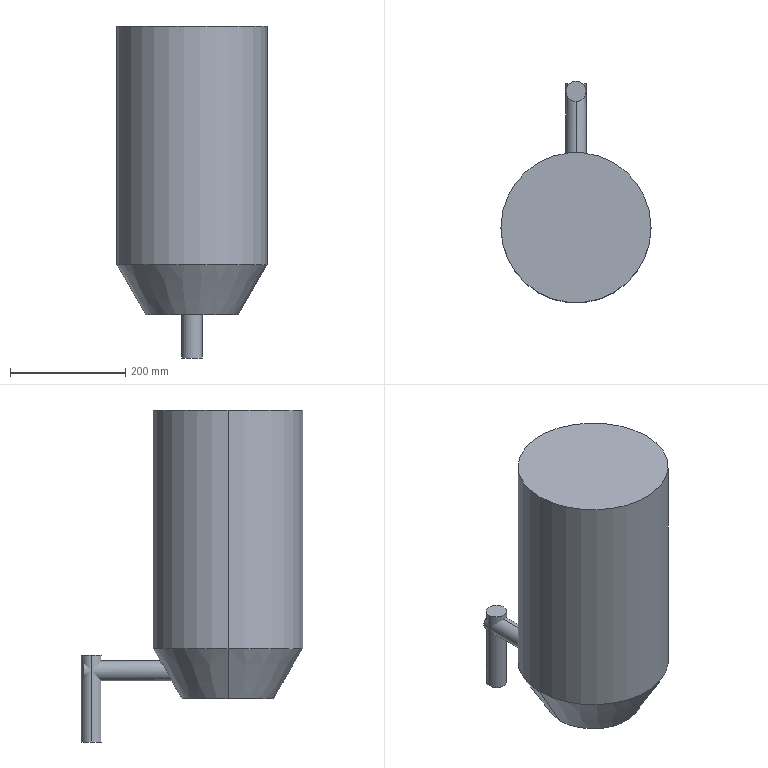Part | STEP file | Vacuum cleaner | 2 solids | 13 faces | box 260 x 384.151 x 575 mm | volume 25286009 mm3 | cylinder 6 | plane 5 | cone 2 | commonest cylinder face diameters 35 x4 260 x2
STEP:
#1=CARTESIAN_POINT('',(0.,250.,66.023));
#2=VERTEX_POINT('',#1);
#3=CARTESIAN_POINT('',(0.,250.,31.023));
#4=VERTEX_POINT('',#3);
#5=CARTESIAN_POINT('',(0.,250.,48.523));
#6=DIRECTION('',(0.,1.,0.));
#7=DIRECTION('',(0.,0.,1.));
#8=AXIS2_PLACEMENT_3D('',#5,#6,#7);
#9=CIRCLE('',#8,17.5);
#10=EDGE_CURVE('',#2,#4,#9,.T.);
#11=ORIENTED_EDGE('',*,*,#10,.F.);
#12=CARTESIAN_POINT('',(0.,118.118,66.023));
#13=VERTEX_POINT('',#12);
#14=CARTESIAN_POINT('',(0.,250.,66.023));
#15=DIRECTION('',(0.,-1.,0.));
#16=VECTOR('',#15,1000.);
#17=LINE('',#14,#16);
#18=EDGE_CURVE('',#2,#13,#17,.T.);
#19=ORIENTED_EDGE('',*,*,#18,.T.);
#20=CARTESIAN_POINT('',(0.,97.911,31.023));
#21=VERTEX_POINT('',#20);
#22=CARTESIAN_POINT('',(0.,97.911,31.023));
#23=CARTESIAN_POINT('',(0.3117,97.911,31.023));
#24=CARTESIAN_POINT('',(0.6247,97.914,31.031));
#25=CARTESIAN_POINT('',(1.245,97.928,31.064));
#26=CARTESIAN_POINT('',(1.554,97.937,31.089));
#27=CARTESIAN_POINT('',(2.475,97.977,31.187));
#28=CARTESIAN_POINT('',(3.082,98.016,31.285));
#29=CARTESIAN_POINT('',(4.284,98.12,31.544));
#30=CARTESIAN_POINT('',(4.878,98.185,31.705));
#31=CARTESIAN_POINT('',(6.054,98.344,32.092));
#32=CARTESIAN_POINT('',(6.629,98.436,32.315));
#33=CARTESIAN_POINT('',(8.295,98.749,33.065));
#34=CARTESIAN_POINT('',(9.338,99.006,33.673));
#35=CARTESIAN_POINT('',(10.803,99.474,34.742));
#36=CARTESIAN_POINT('',(11.268,99.642,35.12));
#37=CARTESIAN_POINT('',(12.148,99.999,35.912));
#38=CARTESIAN_POINT('',(12.563,100.189,36.326));
#39=CARTESIAN_POINT('',(13.348,100.591,37.191));
#40=CARTESIAN_POINT('',(13.718,100.803,37.641));
#41=CARTESIAN_POINT('',(14.41,101.252,38.575));
#42=CARTESIAN_POINT('',(14.73,101.486,39.056));
#43=CARTESIAN_POINT('',(15.606,102.212,40.522));
#44=CARTESIAN_POINT('',(16.083,102.73,41.536));
#45=CARTESIAN_POINT('',(16.65,103.557,43.106));
#46=CARTESIAN_POINT('',(16.814,103.842,43.638));
#47=CARTESIAN_POINT('',(17.086,104.419,44.701));
#48=CARTESIAN_POINT('',(17.197,104.713,45.233));
#49=CARTESIAN_POINT('',(17.452,105.607,46.833));
#50=CARTESIAN_POINT('',(17.522,106.221,47.903));
#51=CARTESIAN_POINT('',(17.466,107.487,50.051));
#52=CARTESIAN_POINT('',(17.341,108.123,51.102));
#53=CARTESIAN_POINT('',(16.906,109.396,53.164));
#54=CARTESIAN_POINT('',(16.597,110.034,54.175));
#55=CARTESIAN_POINT('',(15.784,111.309,56.156));
#56=CARTESIAN_POINT('',(15.29,111.93,57.102));
#57=CARTESIAN_POINT('',(14.13,113.13,58.903));
#58=CARTESIAN_POINT('',(13.463,113.71,59.758));
#59=CARTESIAN_POINT('',(12.316,114.54,60.967));
#60=CARTESIAN_POINT('',(11.908,114.81,61.359));
#61=CARTESIAN_POINT('',(11.057,115.325,62.099));
#62=CARTESIAN_POINT('',(10.612,115.57,62.45));
#63=CARTESIAN_POINT('',(9.682,116.035,63.112));
#64=CARTESIAN_POINT('',(9.196,116.255,63.423));
#65=CARTESIAN_POINT('',(8.181,116.667,64.004));
#66=CARTESIAN_POINT('',(7.648,116.86,64.274));
#67=CARTESIAN_POINT('',(6.013,117.379,65.));
#68=CARTESIAN_POINT('',(4.874,117.649,65.374));
#69=CARTESIAN_POINT('',(3.385,117.881,65.695));
#70=CARTESIAN_POINT('',(3.084,117.922,65.752));
#71=CARTESIAN_POINT('',(2.475,117.993,65.85));
#72=CARTESIAN_POINT('',(2.165,118.023,65.891));
#73=CARTESIAN_POINT('',(1.235,118.095,65.99));
#74=CARTESIAN_POINT('',(0.617,118.118,66.023));
#75=CARTESIAN_POINT('',(0.,118.118,66.023));
#76=B_SPLINE_CURVE_WITH_KNOTS('',3,(#22,#23,#24,#25,#26,#27,#28,#29,#30,#31,#32,#33,#34,#35,#36,#37,#38,#39,#40,#41,#42,#43,#44,#45,#46,#47,#48,#49,#50,#51,#52,#53,#54,#55,#56,#57,#58,#59,#60,#61,#62,#63,#64,#65,#66,#67,#68,#69,#70,#71,#72,#73,#74,#75),.UNSPECIFIED.,.F.,.F.,(4,2,2,2,2,2,2,2,2,2,2,2,2,2,2,2,2,2,2,2,2,2,2,2,2,2,4),(0.01089,0.01181,0.01274,0.01459,0.01644,0.01828,0.02198,0.02383,0.02568,0.02753,0.02938,0.03308,0.03493,0.03678,0.04047,0.04417,0.04787,0.05157,0.05527,0.05712,0.05896,0.06081,0.06266,0.06636,0.06729,0.06821,0.07006),.UNSPECIFIED.);
#77=EDGE_CURVE('',#21,#13,#76,.T.);
#78=ORIENTED_EDGE('',*,*,#77,.F.);
#79=CARTESIAN_POINT('',(0.,250.,31.023));
#80=DIRECTION('',(0.,-1.,0.));
#81=VECTOR('',#80,1000.);
#82=LINE('',#79,#81);
#83=EDGE_CURVE('',#4,#21,#82,.T.);
#84=ORIENTED_EDGE('',*,*,#83,.F.);
#85=EDGE_LOOP('',(#11,#19,#78,#84));
#86=FACE_OUTER_BOUND('',#85,.T.);
#87=CARTESIAN_POINT('',(0.,250.,48.523));
#88=DIRECTION('',(0.,-1.,0.));
#89=DIRECTION('',(0.,0.,-1.));
#90=AXIS2_PLACEMENT_3D('',#87,#88,#89);
#91=CYLINDRICAL_SURFACE('',#90,17.5);
#92=ADVANCED_FACE('',(#86),#91,.T.);
#93=CARTESIAN_POINT('',(130.,0.,500.));
#94=VERTEX_POINT('',#93);
#95=CARTESIAN_POINT('',(-130.,0.,500.));
#96=VERTEX_POINT('',#95);
#97=CARTESIAN_POINT('',(0.,0.,500.));
#98=DIRECTION('',(0.,0.,1.));
#99=DIRECTION('',(1.,0.,0.));
#100=AXIS2_PLACEMENT_3D('',#97,#98,#99);
#101=CIRCLE('',#100,130.);
#102=EDGE_CURVE('',#94,#96,#101,.T.);
#103=ORIENTED_EDGE('',*,*,#102,.F.);
#104=CARTESIAN_POINT('',(130.,0.,86.603));
#105=VERTEX_POINT('',#104);
#106=CARTESIAN_POINT('',(130.,0.,500.));
#107=DIRECTION('',(0.,0.,-1.));
#108=VECTOR('',#107,1000.);
#109=LINE('',#106,#108);
#110=EDGE_CURVE('',#94,#105,#109,.T.);
#111=ORIENTED_EDGE('',*,*,#110,.T.);
#112=CARTESIAN_POINT('',(-130.,0.,86.603));
#113=VERTEX_POINT('',#112);
#114=CARTESIAN_POINT('',(0.,0.,86.603));
#115=DIRECTION('',(0.,0.,1.));
#116=DIRECTION('',(1.,0.,0.));
#117=AXIS2_PLACEMENT_3D('',#114,#115,#116);
#118=CIRCLE('',#117,130.);
#119=EDGE_CURVE('',#105,#113,#118,.T.);
#120=ORIENTED_EDGE('',*,*,#119,.T.);
#121=CARTESIAN_POINT('',(-130.,0.,500.));
#122=DIRECTION('',(0.,0.,-1.));
#123=VECTOR('',#122,1000.);
#124=LINE('',#121,#123);
#125=EDGE_CURVE('',#96,#113,#124,.T.);
#126=ORIENTED_EDGE('',*,*,#125,.F.);
#127=EDGE_LOOP('',(#103,#111,#120,#126));
#128=FACE_OUTER_BOUND('',#127,.T.);
#129=CARTESIAN_POINT('',(0.,0.,500.));
#130=DIRECTION('',(0.,0.,-1.));
#131=DIRECTION('',(-1.,0.,0.));
#132=AXIS2_PLACEMENT_3D('',#129,#130,#131);
#133=CYLINDRICAL_SURFACE('',#132,130.);
#134=ADVANCED_FACE('',(#128),#133,.T.);
#135=ORIENTED_EDGE('',*,*,#77,.T.);
#136=CARTESIAN_POINT('',(0.,118.118,66.023));
#137=CARTESIAN_POINT('',(-0.6162,118.118,66.023));
#138=CARTESIAN_POINT('',(-1.231,118.095,65.99));
#139=CARTESIAN_POINT('',(-2.151,118.024,65.893));
#140=CARTESIAN_POINT('',(-2.457,117.995,65.852));
#141=CARTESIAN_POINT('',(-3.069,117.924,65.754));
#142=CARTESIAN_POINT('',(-3.375,117.882,65.697));
#143=CARTESIAN_POINT('',(-4.878,117.649,65.374));
#144=CARTESIAN_POINT('',(-6.024,117.377,64.997));
#145=CARTESIAN_POINT('',(-7.39,116.942,64.389));
#146=CARTESIAN_POINT('',(-7.66,116.85,64.26));
#147=CARTESIAN_POINT('',(-8.189,116.659,63.991));
#148=CARTESIAN_POINT('',(-8.448,116.559,63.852));
#149=CARTESIAN_POINT('',(-9.208,116.25,63.416));
#150=CARTESIAN_POINT('',(-9.694,116.029,63.103));
#151=CARTESIAN_POINT('',(-10.628,115.562,62.438));
#152=CARTESIAN_POINT('',(-11.075,115.315,62.085));
#153=CARTESIAN_POINT('',(-11.931,114.796,61.338));
#154=CARTESIAN_POINT('',(-12.334,114.527,60.949));
#155=CARTESIAN_POINT('',(-13.476,113.699,59.742));
#156=CARTESIAN_POINT('',(-14.146,113.116,58.882));
#157=CARTESIAN_POINT('',(-15.025,112.203,57.511));
#158=CARTESIAN_POINT('',(-15.296,111.893,57.041));
#159=CARTESIAN_POINT('',(-15.788,111.27,56.091));
#160=CARTESIAN_POINT('',(-16.011,110.956,55.607));
#161=CARTESIAN_POINT('',(-16.609,110.009,54.135));
#162=CARTESIAN_POINT('',(-16.918,109.37,53.123));
#163=CARTESIAN_POINT('',(-17.352,108.081,51.034));
#164=CARTESIAN_POINT('',(-17.471,107.444,49.979));
#165=CARTESIAN_POINT('',(-17.52,106.197,47.86));
#166=CARTESIAN_POINT('',(-17.448,105.584,46.794));
#167=CARTESIAN_POINT('',(-17.187,104.685,45.182));
#168=CARTESIAN_POINT('',(-17.073,104.388,44.643));
#169=CARTESIAN_POINT('',(-16.797,103.813,43.583));
#170=CARTESIAN_POINT('',(-16.634,103.533,43.059));
#171=CARTESIAN_POINT('',(-16.07,102.716,41.508));
#172=CARTESIAN_POINT('',(-15.595,102.201,40.5));
#173=CARTESIAN_POINT('',(-14.715,101.475,39.033));
#174=CARTESIAN_POINT('',(-14.392,101.239,38.549));
#175=CARTESIAN_POINT('',(-13.7,100.793,37.619));
#176=CARTESIAN_POINT('',(-13.331,100.581,37.17));
#177=CARTESIAN_POINT('',(-12.154,99.981,35.878));
#178=CARTESIAN_POINT('',(-11.278,99.625,35.087));
#179=CARTESIAN_POINT('',(-9.321,99.002,33.663));
#180=CARTESIAN_POINT('',(-8.276,98.744,33.056));
#181=CARTESIAN_POINT('',(-6.614,98.433,32.309));
#182=CARTESIAN_POINT('',(-6.044,98.342,32.088));
#183=CARTESIAN_POINT('',(-4.87,98.184,31.702));
#184=CARTESIAN_POINT('',(-4.272,98.119,31.541));
#185=CARTESIAN_POINT('',(-2.469,97.963,31.154));
#186=CARTESIAN_POINT('',(-1.245,97.911,31.023));
#187=CARTESIAN_POINT('',(0.,97.911,31.023));
#188=B_SPLINE_CURVE_WITH_KNOTS('',3,(#136,#137,#138,#139,#140,#141,#142,#143,#144,#145,#146,#147,#148,#149,#150,#151,#152,#153,#154,#155,#156,#157,#158,#159,#160,#161,#162,#163,#164,#165,#166,#167,#168,#169,#170,#171,#172,#173,#174,#175,#176,#177,#178,#179,#180,#181,#182,#183,#184,#185,#186,#187),.UNSPECIFIED.,.F.,.F.,(4,2,2,2,2,2,2,2,2,2,2,2,2,2,2,2,2,2,2,2,2,2,2,2,2,4),(0.07006,0.07191,0.07283,0.07375,0.07745,0.07837,0.07929,0.08114,0.08299,0.08483,0.08853,0.09037,0.09222,0.09591,0.09961,0.1033,0.1051,0.107,0.1107,0.1125,0.1144,0.1181,0.1218,0.1236,0.1255,0.1292),.UNSPECIFIED.);
#189=EDGE_CURVE('',#13,#21,#188,.T.);
#190=ORIENTED_EDGE('',*,*,#189,.T.);
#191=EDGE_LOOP('',(#135,#190));
#192=FACE_BOUND('',#191,.T.);
#193=CARTESIAN_POINT('',(-80.,0.,0.));
#194=VERTEX_POINT('',#193);
#195=CARTESIAN_POINT('',(80.,0.,0.));
#196=VERTEX_POINT('',#195);
#197=CARTESIAN_POINT('',(0.,0.,0.));
#198=DIRECTION('',(0.,0.,-1.));
#199=DIRECTION('',(1.,0.,0.));
#200=AXIS2_PLACEMENT_3D('',#197,#198,#199);
#201=CIRCLE('',#200,80.);
#202=EDGE_CURVE('',#194,#196,#201,.T.);
#203=ORIENTED_EDGE('',*,*,#202,.F.);
#204=CARTESIAN_POINT('',(-130.,0.,86.603));
#205=DIRECTION('',(-0.5,0.,0.866));
#206=VECTOR('',#205,1000.);
#207=LINE('',#204,#206);
#208=EDGE_CURVE('',#194,#113,#207,.T.);
#209=ORIENTED_EDGE('',*,*,#208,.T.);
#210=ORIENTED_EDGE('',*,*,#119,.F.);
#211=CARTESIAN_POINT('',(130.,0.,86.603));
#212=DIRECTION('',(0.5,0.,0.866));
#213=VECTOR('',#212,1000.);
#214=LINE('',#211,#213);
#215=EDGE_CURVE('',#196,#105,#214,.T.);
#216=ORIENTED_EDGE('',*,*,#215,.F.);
#217=EDGE_LOOP('',(#203,#209,#210,#216));
#218=FACE_OUTER_BOUND('',#217,.T.);
#219=CARTESIAN_POINT('',(0.,0.,86.603));
#220=DIRECTION('',(0.,0.,1.));
#221=DIRECTION('',(1.,0.,0.));
#222=AXIS2_PLACEMENT_3D('',#219,#220,#221);
#223=CONICAL_SURFACE('',#222,130.,0.5236);
#224=ADVANCED_FACE('',(#192,#218),#223,.T.);
#225=ORIENTED_EDGE('',*,*,#208,.F.);
#226=CARTESIAN_POINT('',(0.,0.,0.));
#227=DIRECTION('',(0.,0.,-1.));
#228=DIRECTION('',(1.,0.,0.));
#229=AXIS2_PLACEMENT_3D('',#226,#227,#228);
#230=CIRCLE('',#229,80.);
#231=EDGE_CURVE('',#196,#194,#230,.T.);
#232=ORIENTED_EDGE('',*,*,#231,.F.);
#233=ORIENTED_EDGE('',*,*,#215,.T.);
#234=CARTESIAN_POINT('',(0.,0.,86.603));
#235=DIRECTION('',(0.,0.,1.));
#236=DIRECTION('',(1.,0.,0.));
#237=AXIS2_PLACEMENT_3D('',#234,#235,#236);
#238=CIRCLE('',#237,130.);
#239=EDGE_CURVE('',#113,#105,#238,.T.);
#240=ORIENTED_EDGE('',*,*,#239,.F.);
#241=EDGE_LOOP('',(#225,#232,#233,#240));
#242=FACE_OUTER_BOUND('',#241,.T.);
#243=CARTESIAN_POINT('',(0.,0.,86.603));
#244=DIRECTION('',(0.,0.,1.));
#245=DIRECTION('',(1.,0.,0.));
#246=AXIS2_PLACEMENT_3D('',#243,#244,#245);
#247=CONICAL_SURFACE('',#246,130.,0.5236);
#248=ADVANCED_FACE('',(#242),#247,.T.);
#249=ORIENTED_EDGE('',*,*,#110,.F.);
#250=CARTESIAN_POINT('',(0.,0.,500.));
#251=DIRECTION('',(0.,0.,1.));
#252=DIRECTION('',(1.,0.,0.));
#253=AXIS2_PLACEMENT_3D('',#250,#251,#252);
#254=CIRCLE('',#253,130.);
#255=EDGE_CURVE('',#96,#94,#254,.T.);
#256=ORIENTED_EDGE('',*,*,#255,.F.);
#257=ORIENTED_EDGE('',*,*,#125,.T.);
#258=ORIENTED_EDGE('',*,*,#239,.T.);
#259=EDGE_LOOP('',(#249,#256,#257,#258));
#260=FACE_OUTER_BOUND('',#259,.T.);
#261=CARTESIAN_POINT('',(0.,0.,500.));
#262=DIRECTION('',(0.,0.,-1.));
#263=DIRECTION('',(-1.,0.,0.));
#264=AXIS2_PLACEMENT_3D('',#261,#262,#263);
#265=CYLINDRICAL_SURFACE('',#264,130.);
#266=ADVANCED_FACE('',(#260),#265,.T.);
#267=ORIENTED_EDGE('',*,*,#255,.T.);
#268=ORIENTED_EDGE('',*,*,#102,.T.);
#269=EDGE_LOOP('',(#267,#268));
#270=FACE_OUTER_BOUND('',#269,.T.);
#271=CARTESIAN_POINT('',(0.,0.,500.));
#272=DIRECTION('',(0.,0.,1.));
#273=DIRECTION('',(1.,0.,0.));
#274=AXIS2_PLACEMENT_3D('',#271,#272,#273);
#275=PLANE('',#274);
#276=ADVANCED_FACE('',(#270),#275,.T.);
#277=ORIENTED_EDGE('',*,*,#231,.T.);
#278=ORIENTED_EDGE('',*,*,#202,.T.);
#279=EDGE_LOOP('',(#277,#278));
#280=FACE_OUTER_BOUND('',#279,.T.);
#281=CARTESIAN_POINT('',(0.,0.,0.));
#282=DIRECTION('',(0.,0.,1.));
#283=DIRECTION('',(1.,0.,0.));
#284=AXIS2_PLACEMENT_3D('',#281,#282,#283);
#285=PLANE('',#284);
#286=ADVANCED_FACE('',(#280),#285,.F.);
#287=ORIENTED_EDGE('',*,*,#18,.F.);
#288=CARTESIAN_POINT('',(0.,250.,48.523));
#289=DIRECTION('',(0.,1.,0.));
#290=DIRECTION('',(0.,0.,1.));
#291=AXIS2_PLACEMENT_3D('',#288,#289,#290);
#292=CIRCLE('',#291,17.5);
#293=EDGE_CURVE('',#4,#2,#292,.T.);
#294=ORIENTED_EDGE('',*,*,#293,.F.);
#295=ORIENTED_EDGE('',*,*,#83,.T.);
#296=ORIENTED_EDGE('',*,*,#189,.F.);
#297=EDGE_LOOP('',(#287,#294,#295,#296));
#298=FACE_OUTER_BOUND('',#297,.T.);
#299=CARTESIAN_POINT('',(0.,250.,48.523));
#300=DIRECTION('',(0.,-1.,0.));
#301=DIRECTION('',(0.,0.,-1.));
#302=AXIS2_PLACEMENT_3D('',#299,#300,#301);
#303=CYLINDRICAL_SURFACE('',#302,17.5);
#304=ADVANCED_FACE('',(#298),#303,.T.);
#305=ORIENTED_EDGE('',*,*,#293,.T.);
#306=ORIENTED_EDGE('',*,*,#10,.T.);
#307=EDGE_LOOP('',(#305,#306));
#308=FACE_OUTER_BOUND('',#307,.T.);
#309=CARTESIAN_POINT('',(0.,250.,48.523));
#310=DIRECTION('',(0.,1.,0.));
#311=DIRECTION('',(0.,0.,1.));
#312=AXIS2_PLACEMENT_3D('',#309,#310,#311);
#313=PLANE('',#312);
#314=ADVANCED_FACE('',(#308),#313,.T.);
#315=CLOSED_SHELL('',(#92,#134,#224,#248,#266,#276,#286,#304,#314));
#316=MANIFOLD_SOLID_BREP('',#315);
#317=CARTESIAN_POINT('',(17.5,236.651,-75.));
#318=VERTEX_POINT('',#317);
#319=CARTESIAN_POINT('',(-17.5,236.651,-75.));
#320=VERTEX_POINT('',#319);
#321=CARTESIAN_POINT('',(0.,236.651,-75.));
#322=DIRECTION('',(0.,0.,1.));
#323=DIRECTION('',(1.,0.,0.));
#324=AXIS2_PLACEMENT_3D('',#321,#322,#323);
#325=CIRCLE('',#324,17.5);
#326=EDGE_CURVE('',#318,#320,#325,.T.);
#327=ORIENTED_EDGE('',*,*,#326,.T.);
#328=CARTESIAN_POINT('',(-17.5,236.651,75.));
#329=VERTEX_POINT('',#328);
#330=CARTESIAN_POINT('',(-17.5,236.651,-75.));
#331=DIRECTION('',(0.,0.,1.));
#332=VECTOR('',#331,1000.);
#333=LINE('',#330,#332);
#334=EDGE_CURVE('',#320,#329,#333,.T.);
#335=ORIENTED_EDGE('',*,*,#334,.T.);
#336=CARTESIAN_POINT('',(17.5,236.651,75.));
#337=VERTEX_POINT('',#336);
#338=CARTESIAN_POINT('',(0.,236.651,75.));
#339=DIRECTION('',(0.,0.,1.));
#340=DIRECTION('',(1.,0.,0.));
#341=AXIS2_PLACEMENT_3D('',#338,#339,#340);
#342=CIRCLE('',#341,17.5);
#343=EDGE_CURVE('',#337,#329,#342,.T.);
#344=ORIENTED_EDGE('',*,*,#343,.F.);
#345=CARTESIAN_POINT('',(17.5,236.651,-75.));
#346=DIRECTION('',(0.,0.,1.));
#347=VECTOR('',#346,1000.);
#348=LINE('',#345,#347);
#349=EDGE_CURVE('',#318,#337,#348,.T.);
#350=ORIENTED_EDGE('',*,*,#349,.F.);
#351=EDGE_LOOP('',(#327,#335,#344,#350));
#352=FACE_OUTER_BOUND('',#351,.T.);
#353=CARTESIAN_POINT('',(0.,236.651,-75.));
#354=DIRECTION('',(0.,0.,1.));
#355=DIRECTION('',(1.,0.,0.));
#356=AXIS2_PLACEMENT_3D('',#353,#354,#355);
#357=CYLINDRICAL_SURFACE('',#356,17.5);
#358=ADVANCED_FACE('',(#352),#357,.T.);
#359=ORIENTED_EDGE('',*,*,#334,.F.);
#360=CARTESIAN_POINT('',(0.,236.651,-75.));
#361=DIRECTION('',(0.,0.,1.));
#362=DIRECTION('',(1.,0.,0.));
#363=AXIS2_PLACEMENT_3D('',#360,#361,#362);
#364=CIRCLE('',#363,17.5);
#365=EDGE_CURVE('',#320,#318,#364,.T.);
#366=ORIENTED_EDGE('',*,*,#365,.T.);
#367=ORIENTED_EDGE('',*,*,#349,.T.);
#368=CARTESIAN_POINT('',(0.,236.651,75.));
#369=DIRECTION('',(0.,0.,1.));
#370=DIRECTION('',(1.,0.,0.));
#371=AXIS2_PLACEMENT_3D('',#368,#369,#370);
#372=CIRCLE('',#371,17.5);
#373=EDGE_CURVE('',#329,#337,#372,.T.);
#374=ORIENTED_EDGE('',*,*,#373,.F.);
#375=EDGE_LOOP('',(#359,#366,#367,#374));
#376=FACE_OUTER_BOUND('',#375,.T.);
#377=CARTESIAN_POINT('',(0.,236.651,-75.));
#378=DIRECTION('',(0.,0.,1.));
#379=DIRECTION('',(1.,0.,0.));
#380=AXIS2_PLACEMENT_3D('',#377,#378,#379);
#381=CYLINDRICAL_SURFACE('',#380,17.5);
#382=ADVANCED_FACE('',(#376),#381,.T.);
#383=ORIENTED_EDGE('',*,*,#326,.F.);
#384=ORIENTED_EDGE('',*,*,#365,.F.);
#385=EDGE_LOOP('',(#383,#384));
#386=FACE_OUTER_BOUND('',#385,.T.);
#387=CARTESIAN_POINT('',(0.,236.651,-75.));
#388=DIRECTION('',(0.,0.,1.));
#389=DIRECTION('',(1.,0.,0.));
#390=AXIS2_PLACEMENT_3D('',#387,#388,#389);
#391=PLANE('',#390);
#392=ADVANCED_FACE('',(#386),#391,.F.);
#393=ORIENTED_EDGE('',*,*,#343,.T.);
#394=ORIENTED_EDGE('',*,*,#373,.T.);
#395=EDGE_LOOP('',(#393,#394));
#396=FACE_OUTER_BOUND('',#395,.T.);
#397=CARTESIAN_POINT('',(0.,236.651,75.));
#398=DIRECTION('',(0.,0.,1.));
#399=DIRECTION('',(1.,0.,0.));
#400=AXIS2_PLACEMENT_3D('',#397,#398,#399);
#401=PLANE('',#400);
#402=ADVANCED_FACE('',(#396),#401,.T.);
#403=CLOSED_SHELL('',(#358,#382,#392,#402));
#404=MANIFOLD_SOLID_BREP('',#403);
#405=CARTESIAN_POINT('',(0.,0.,0.));
#406=DIRECTION('',(0.,0.,1.));
#407=DIRECTION('',(1.,0.,0.));
#408=AXIS2_PLACEMENT_3D('',#405,#406,#407);
#409=(LENGTH_UNIT()NAMED_UNIT(*)SI_UNIT(.MILLI.,.METRE.));
#410=UNCERTAINTY_MEASURE_WITH_UNIT(LENGTH_MEASURE(0.00001),#409,'','');
#411=(NAMED_UNIT(*)PLANE_ANGLE_UNIT()SI_UNIT($,.RADIAN.));
#412=(NAMED_UNIT(*)SI_UNIT($,.STERADIAN.)SOLID_ANGLE_UNIT());
#413=(GEOMETRIC_REPRESENTATION_CONTEXT(3)GLOBAL_UNCERTAINTY_ASSIGNED_CONTEXT((#410))GLOBAL_UNIT_ASSIGNED_CONTEXT((#409,#411,#412))REPRESENTATION_CONTEXT('',''));
#414=ADVANCED_BREP_SHAPE_REPRESENTATION('',(#316,#404,#408),#413);